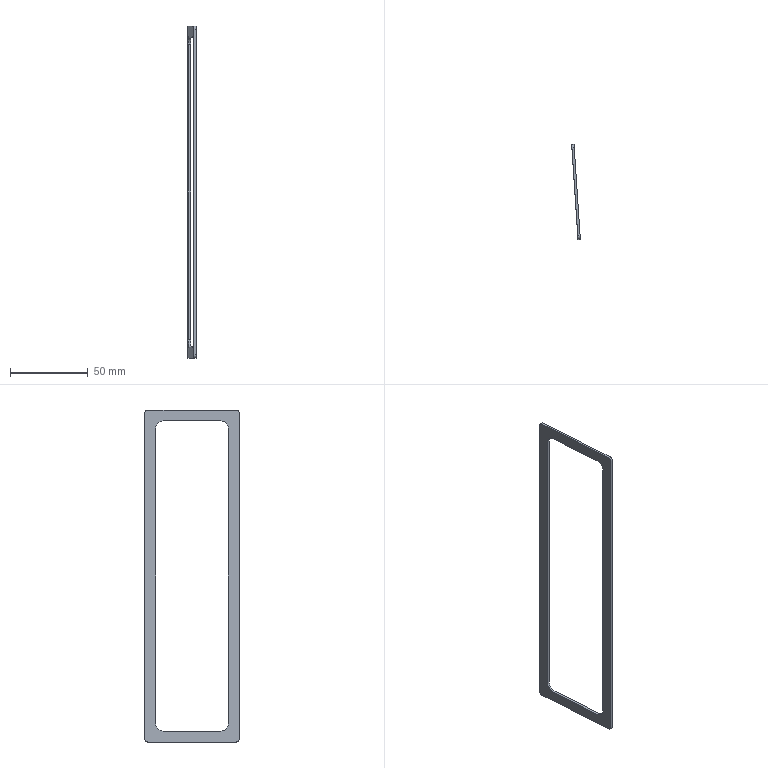Part | SolidWorks | features BaseBody 1 | 1 solid | 18 faces | box 5.536 x 60.965 x 214 mm | volume 5508 mm3 | plane 10 | cylinder 8 | commonest cylinder face diameters 4 x4 10 x4
STEP:
#1=CARTESIAN_POINT('',(-18.857,44.213,71.25));
#2=VERTEX_POINT('',#1);
#3=CARTESIAN_POINT('',(-18.857,44.213,-118.75));
#4=VERTEX_POINT('',#3);
#5=CARTESIAN_POINT('',(-18.857,44.213,-118.75));
#6=DIRECTION('',(0.,0.,-1.));
#7=VECTOR('',#6,1000.);
#8=LINE('',#5,#7);
#9=EDGE_CURVE('',#2,#4,#8,.T.);
#10=ORIENTED_EDGE('',*,*,#9,.F.);
#11=CARTESIAN_POINT('',(-20.353,44.113,71.25));
#12=VERTEX_POINT('',#11);
#13=CARTESIAN_POINT('',(-20.353,44.113,71.25));
#14=DIRECTION('',(0.9978,0.06623,0.));
#15=VECTOR('',#14,1000.);
#16=LINE('',#13,#15);
#17=EDGE_CURVE('',#12,#2,#16,.T.);
#18=ORIENTED_EDGE('',*,*,#17,.F.);
#19=CARTESIAN_POINT('',(-20.353,44.113,-118.75));
#20=VERTEX_POINT('',#19);
#21=CARTESIAN_POINT('',(-20.353,44.113,-118.75));
#22=DIRECTION('',(0.,0.,-1.));
#23=VECTOR('',#22,1000.);
#24=LINE('',#21,#23);
#25=EDGE_CURVE('',#12,#20,#24,.T.);
#26=ORIENTED_EDGE('',*,*,#25,.T.);
#27=CARTESIAN_POINT('',(-20.353,44.113,-118.75));
#28=DIRECTION('',(0.9978,0.06623,0.));
#29=VECTOR('',#28,1000.);
#30=LINE('',#27,#29);
#31=EDGE_CURVE('',#20,#4,#30,.T.);
#32=ORIENTED_EDGE('',*,*,#31,.T.);
#33=EDGE_LOOP('',(#10,#18,#26,#32));
#34=FACE_OUTER_BOUND('',#33,.T.);
#35=CARTESIAN_POINT('',(-20.353,44.113,-118.75));
#36=DIRECTION('',(0.06623,-0.9978,0.));
#37=DIRECTION('',(0.,0.,-1.));
#38=AXIS2_PLACEMENT_3D('',#35,#36,#37);
#39=PLANE('',#38);
#40=ADVANCED_FACE('',(#34),#39,.T.);
#41=CARTESIAN_POINT('',(-18.526,39.224,76.25));
#42=VERTEX_POINT('',#41);
#43=CARTESIAN_POINT('',(-18.526,39.224,71.25));
#44=DIRECTION('',(-0.9978,-0.06623,0.));
#45=DIRECTION('',(0.,0.,-1.));
#46=AXIS2_PLACEMENT_3D('',#43,#44,#45);
#47=CIRCLE('',#46,5.);
#48=EDGE_CURVE('',#42,#2,#47,.T.);
#49=ORIENTED_EDGE('',*,*,#48,.F.);
#50=CARTESIAN_POINT('',(-20.022,39.124,76.25));
#51=VERTEX_POINT('',#50);
#52=CARTESIAN_POINT('',(-20.022,39.124,76.25));
#53=DIRECTION('',(0.9978,0.06623,0.));
#54=VECTOR('',#53,1000.);
#55=LINE('',#52,#54);
#56=EDGE_CURVE('',#51,#42,#55,.T.);
#57=ORIENTED_EDGE('',*,*,#56,.F.);
#58=CARTESIAN_POINT('',(-20.022,39.124,71.25));
#59=DIRECTION('',(-0.9978,-0.06623,0.));
#60=DIRECTION('',(0.,0.,-1.));
#61=AXIS2_PLACEMENT_3D('',#58,#59,#60);
#62=CIRCLE('',#61,5.);
#63=EDGE_CURVE('',#51,#12,#62,.T.);
#64=ORIENTED_EDGE('',*,*,#63,.T.);
#65=ORIENTED_EDGE('',*,*,#17,.T.);
#66=EDGE_LOOP('',(#49,#57,#64,#65));
#67=FACE_OUTER_BOUND('',#66,.T.);
#68=CARTESIAN_POINT('',(-20.022,39.124,71.25));
#69=DIRECTION('',(0.9978,0.06623,0.));
#70=DIRECTION('',(0.,0.,-1.));
#71=AXIS2_PLACEMENT_3D('',#68,#69,#70);
#72=CYLINDRICAL_SURFACE('',#71,5.);
#73=ADVANCED_FACE('',(#67),#72,.F.);
#74=CARTESIAN_POINT('',(-16.075,2.305,76.25));
#75=VERTEX_POINT('',#74);
#76=CARTESIAN_POINT('',(-18.526,39.224,76.25));
#77=DIRECTION('',(-0.06623,0.9978,0.));
#78=VECTOR('',#77,1000.);
#79=LINE('',#76,#78);
#80=EDGE_CURVE('',#75,#42,#79,.T.);
#81=ORIENTED_EDGE('',*,*,#80,.F.);
#82=CARTESIAN_POINT('',(-17.572,2.206,76.25));
#83=VERTEX_POINT('',#82);
#84=CARTESIAN_POINT('',(-17.572,2.206,76.25));
#85=DIRECTION('',(0.9978,0.06623,0.));
#86=VECTOR('',#85,1000.);
#87=LINE('',#84,#86);
#88=EDGE_CURVE('',#83,#75,#87,.T.);
#89=ORIENTED_EDGE('',*,*,#88,.F.);
#90=CARTESIAN_POINT('',(-20.022,39.124,76.25));
#91=DIRECTION('',(-0.06623,0.9978,0.));
#92=VECTOR('',#91,1000.);
#93=LINE('',#90,#92);
#94=EDGE_CURVE('',#83,#51,#93,.T.);
#95=ORIENTED_EDGE('',*,*,#94,.T.);
#96=ORIENTED_EDGE('',*,*,#56,.T.);
#97=EDGE_LOOP('',(#81,#89,#95,#96));
#98=FACE_OUTER_BOUND('',#97,.T.);
#99=CARTESIAN_POINT('',(-20.022,39.124,76.25));
#100=DIRECTION('',(0.,0.,-1.));
#101=DIRECTION('',(-1.,0.,0.));
#102=AXIS2_PLACEMENT_3D('',#99,#100,#101);
#103=PLANE('',#102);
#104=ADVANCED_FACE('',(#98),#103,.T.);
#105=CARTESIAN_POINT('',(-15.744,-2.684,71.25));
#106=VERTEX_POINT('',#105);
#107=CARTESIAN_POINT('',(-16.075,2.305,71.25));
#108=DIRECTION('',(-0.9978,-0.06623,0.));
#109=DIRECTION('',(0.,0.,-1.));
#110=AXIS2_PLACEMENT_3D('',#107,#108,#109);
#111=CIRCLE('',#110,5.);
#112=EDGE_CURVE('',#106,#75,#111,.T.);
#113=ORIENTED_EDGE('',*,*,#112,.F.);
#114=CARTESIAN_POINT('',(-17.241,-2.783,71.25));
#115=VERTEX_POINT('',#114);
#116=CARTESIAN_POINT('',(-17.241,-2.783,71.25));
#117=DIRECTION('',(0.9978,0.06623,0.));
#118=VECTOR('',#117,1000.);
#119=LINE('',#116,#118);
#120=EDGE_CURVE('',#115,#106,#119,.T.);
#121=ORIENTED_EDGE('',*,*,#120,.F.);
#122=CARTESIAN_POINT('',(-17.572,2.206,71.25));
#123=DIRECTION('',(-0.9978,-0.06623,0.));
#124=DIRECTION('',(0.,0.,-1.));
#125=AXIS2_PLACEMENT_3D('',#122,#123,#124);
#126=CIRCLE('',#125,5.);
#127=EDGE_CURVE('',#115,#83,#126,.T.);
#128=ORIENTED_EDGE('',*,*,#127,.T.);
#129=ORIENTED_EDGE('',*,*,#88,.T.);
#130=EDGE_LOOP('',(#113,#121,#128,#129));
#131=FACE_OUTER_BOUND('',#130,.T.);
#132=CARTESIAN_POINT('',(-17.572,2.206,71.25));
#133=DIRECTION('',(0.9978,0.06623,0.));
#134=DIRECTION('',(0.,0.,-1.));
#135=AXIS2_PLACEMENT_3D('',#132,#133,#134);
#136=CYLINDRICAL_SURFACE('',#135,5.);
#137=ADVANCED_FACE('',(#131),#136,.F.);
#138=CARTESIAN_POINT('',(-15.744,-2.684,-118.75));
#139=VERTEX_POINT('',#138);
#140=CARTESIAN_POINT('',(-15.744,-2.684,-118.75));
#141=DIRECTION('',(0.,0.,1.));
#142=VECTOR('',#141,1000.);
#143=LINE('',#140,#142);
#144=EDGE_CURVE('',#139,#106,#143,.T.);
#145=ORIENTED_EDGE('',*,*,#144,.F.);
#146=CARTESIAN_POINT('',(-17.241,-2.783,-118.75));
#147=VERTEX_POINT('',#146);
#148=CARTESIAN_POINT('',(-17.241,-2.783,-118.75));
#149=DIRECTION('',(0.9978,0.06623,0.));
#150=VECTOR('',#149,1000.);
#151=LINE('',#148,#150);
#152=EDGE_CURVE('',#147,#139,#151,.T.);
#153=ORIENTED_EDGE('',*,*,#152,.F.);
#154=CARTESIAN_POINT('',(-17.241,-2.783,-118.75));
#155=DIRECTION('',(0.,0.,1.));
#156=VECTOR('',#155,1000.);
#157=LINE('',#154,#156);
#158=EDGE_CURVE('',#147,#115,#157,.T.);
#159=ORIENTED_EDGE('',*,*,#158,.T.);
#160=ORIENTED_EDGE('',*,*,#120,.T.);
#161=EDGE_LOOP('',(#145,#153,#159,#160));
#162=FACE_OUTER_BOUND('',#161,.T.);
#163=CARTESIAN_POINT('',(-17.241,-2.783,-118.75));
#164=DIRECTION('',(-0.06623,0.9978,0.));
#165=DIRECTION('',(0.,0.,1.));
#166=AXIS2_PLACEMENT_3D('',#163,#164,#165);
#167=PLANE('',#166);
#168=ADVANCED_FACE('',(#162),#167,.T.);
#169=CARTESIAN_POINT('',(-16.075,2.305,-123.75));
#170=VERTEX_POINT('',#169);
#171=CARTESIAN_POINT('',(-16.075,2.305,-118.75));
#172=DIRECTION('',(-0.9978,-0.06623,0.));
#173=DIRECTION('',(0.,0.,-1.));
#174=AXIS2_PLACEMENT_3D('',#171,#172,#173);
#175=CIRCLE('',#174,5.);
#176=EDGE_CURVE('',#170,#139,#175,.T.);
#177=ORIENTED_EDGE('',*,*,#176,.F.);
#178=CARTESIAN_POINT('',(-17.572,2.206,-123.75));
#179=VERTEX_POINT('',#178);
#180=CARTESIAN_POINT('',(-17.572,2.206,-123.75));
#181=DIRECTION('',(0.9978,0.06623,0.));
#182=VECTOR('',#181,1000.);
#183=LINE('',#180,#182);
#184=EDGE_CURVE('',#179,#170,#183,.T.);
#185=ORIENTED_EDGE('',*,*,#184,.F.);
#186=CARTESIAN_POINT('',(-17.572,2.206,-118.75));
#187=DIRECTION('',(-0.9978,-0.06623,0.));
#188=DIRECTION('',(0.,0.,-1.));
#189=AXIS2_PLACEMENT_3D('',#186,#187,#188);
#190=CIRCLE('',#189,5.);
#191=EDGE_CURVE('',#179,#147,#190,.T.);
#192=ORIENTED_EDGE('',*,*,#191,.T.);
#193=ORIENTED_EDGE('',*,*,#152,.T.);
#194=EDGE_LOOP('',(#177,#185,#192,#193));
#195=FACE_OUTER_BOUND('',#194,.T.);
#196=CARTESIAN_POINT('',(-17.572,2.206,-118.75));
#197=DIRECTION('',(0.9978,0.06623,0.));
#198=DIRECTION('',(0.,0.,-1.));
#199=AXIS2_PLACEMENT_3D('',#196,#197,#198);
#200=CYLINDRICAL_SURFACE('',#199,5.);
#201=ADVANCED_FACE('',(#195),#200,.F.);
#202=CARTESIAN_POINT('',(-18.526,39.224,-123.75));
#203=VERTEX_POINT('',#202);
#204=CARTESIAN_POINT('',(-18.526,39.224,-123.75));
#205=DIRECTION('',(0.06623,-0.9978,0.));
#206=VECTOR('',#205,1000.);
#207=LINE('',#204,#206);
#208=EDGE_CURVE('',#203,#170,#207,.T.);
#209=ORIENTED_EDGE('',*,*,#208,.F.);
#210=CARTESIAN_POINT('',(-20.022,39.124,-123.75));
#211=VERTEX_POINT('',#210);
#212=CARTESIAN_POINT('',(-20.022,39.124,-123.75));
#213=DIRECTION('',(0.9978,0.06623,0.));
#214=VECTOR('',#213,1000.);
#215=LINE('',#212,#214);
#216=EDGE_CURVE('',#211,#203,#215,.T.);
#217=ORIENTED_EDGE('',*,*,#216,.F.);
#218=CARTESIAN_POINT('',(-20.022,39.124,-123.75));
#219=DIRECTION('',(0.06623,-0.9978,0.));
#220=VECTOR('',#219,1000.);
#221=LINE('',#218,#220);
#222=EDGE_CURVE('',#211,#179,#221,.T.);
#223=ORIENTED_EDGE('',*,*,#222,.T.);
#224=ORIENTED_EDGE('',*,*,#184,.T.);
#225=EDGE_LOOP('',(#209,#217,#223,#224));
#226=FACE_OUTER_BOUND('',#225,.T.);
#227=CARTESIAN_POINT('',(-20.022,39.124,-123.75));
#228=DIRECTION('',(0.,0.,1.));
#229=DIRECTION('',(1.,0.,0.));
#230=AXIS2_PLACEMENT_3D('',#227,#228,#229);
#231=PLANE('',#230);
#232=ADVANCED_FACE('',(#226),#231,.T.);
#233=CARTESIAN_POINT('',(-18.526,39.224,-118.75));
#234=DIRECTION('',(-0.9978,-0.06623,0.));
#235=DIRECTION('',(0.,0.,1.));
#236=AXIS2_PLACEMENT_3D('',#233,#234,#235);
#237=CIRCLE('',#236,5.);
#238=EDGE_CURVE('',#4,#203,#237,.T.);
#239=ORIENTED_EDGE('',*,*,#238,.F.);
#240=ORIENTED_EDGE('',*,*,#31,.F.);
#241=CARTESIAN_POINT('',(-20.022,39.124,-118.75));
#242=DIRECTION('',(-0.9978,-0.06623,0.));
#243=DIRECTION('',(0.,0.,1.));
#244=AXIS2_PLACEMENT_3D('',#241,#242,#243);
#245=CIRCLE('',#244,5.);
#246=EDGE_CURVE('',#20,#211,#245,.T.);
#247=ORIENTED_EDGE('',*,*,#246,.T.);
#248=ORIENTED_EDGE('',*,*,#216,.T.);
#249=EDGE_LOOP('',(#239,#240,#247,#248));
#250=FACE_OUTER_BOUND('',#249,.T.);
#251=CARTESIAN_POINT('',(-20.022,39.124,-118.75));
#252=DIRECTION('',(0.9978,0.06623,0.));
#253=DIRECTION('',(0.,0.,-1.));
#254=AXIS2_PLACEMENT_3D('',#251,#252,#253);
#255=CYLINDRICAL_SURFACE('',#254,5.);
#256=ADVANCED_FACE('',(#250),#255,.F.);
#257=CARTESIAN_POINT('',(-15.28,-9.669,-128.75));
#258=VERTEX_POINT('',#257);
#259=CARTESIAN_POINT('',(-15.28,-9.669,81.25));
#260=VERTEX_POINT('',#259);
#261=CARTESIAN_POINT('',(-15.28,-9.669,-128.75));
#262=DIRECTION('',(0.,0.,1.));
#263=VECTOR('',#262,1000.);
#264=LINE('',#261,#263);
#265=EDGE_CURVE('',#258,#260,#264,.T.);
#266=ORIENTED_EDGE('',*,*,#265,.T.);
#267=CARTESIAN_POINT('',(-16.777,-9.768,81.25));
#268=VERTEX_POINT('',#267);
#269=CARTESIAN_POINT('',(-16.777,-9.768,81.25));
#270=DIRECTION('',(0.9978,0.06623,0.));
#271=VECTOR('',#270,1000.);
#272=LINE('',#269,#271);
#273=EDGE_CURVE('',#268,#260,#272,.T.);
#274=ORIENTED_EDGE('',*,*,#273,.F.);
#275=CARTESIAN_POINT('',(-16.777,-9.768,-128.75));
#276=VERTEX_POINT('',#275);
#277=CARTESIAN_POINT('',(-16.777,-9.768,-128.75));
#278=DIRECTION('',(0.,0.,1.));
#279=VECTOR('',#278,1000.);
#280=LINE('',#277,#279);
#281=EDGE_CURVE('',#276,#268,#280,.T.);
#282=ORIENTED_EDGE('',*,*,#281,.F.);
#283=CARTESIAN_POINT('',(-16.777,-9.768,-128.75));
#284=DIRECTION('',(0.9978,0.06623,0.));
#285=VECTOR('',#284,1000.);
#286=LINE('',#283,#285);
#287=EDGE_CURVE('',#276,#258,#286,.T.);
#288=ORIENTED_EDGE('',*,*,#287,.T.);
#289=EDGE_LOOP('',(#266,#274,#282,#288));
#290=FACE_OUTER_BOUND('',#289,.T.);
#291=CARTESIAN_POINT('',(-16.777,-9.768,-128.75));
#292=DIRECTION('',(-0.06623,0.9978,0.));
#293=DIRECTION('',(0.,0.,1.));
#294=AXIS2_PLACEMENT_3D('',#291,#292,#293);
#295=PLANE('',#294);
#296=ADVANCED_FACE('',(#290),#295,.F.);
#297=CARTESIAN_POINT('',(-15.413,-7.673,-130.75));
#298=VERTEX_POINT('',#297);
#299=CARTESIAN_POINT('',(-15.413,-7.673,-128.75));
#300=DIRECTION('',(-0.9978,-0.06623,0.));
#301=DIRECTION('',(0.,0.,-1.));
#302=AXIS2_PLACEMENT_3D('',#299,#300,#301);
#303=CIRCLE('',#302,2.);
#304=EDGE_CURVE('',#298,#258,#303,.T.);
#305=ORIENTED_EDGE('',*,*,#304,.T.);
#306=ORIENTED_EDGE('',*,*,#287,.F.);
#307=CARTESIAN_POINT('',(-16.91,-7.772,-130.75));
#308=VERTEX_POINT('',#307);
#309=CARTESIAN_POINT('',(-16.91,-7.772,-128.75));
#310=DIRECTION('',(-0.9978,-0.06623,0.));
#311=DIRECTION('',(0.,0.,-1.));
#312=AXIS2_PLACEMENT_3D('',#309,#310,#311);
#313=CIRCLE('',#312,2.);
#314=EDGE_CURVE('',#308,#276,#313,.T.);
#315=ORIENTED_EDGE('',*,*,#314,.F.);
#316=CARTESIAN_POINT('',(-16.91,-7.772,-130.75));
#317=DIRECTION('',(0.9978,0.06623,0.));
#318=VECTOR('',#317,1000.);
#319=LINE('',#316,#318);
#320=EDGE_CURVE('',#308,#298,#319,.T.);
#321=ORIENTED_EDGE('',*,*,#320,.T.);
#322=EDGE_LOOP('',(#305,#306,#315,#321));
#323=FACE_OUTER_BOUND('',#322,.T.);
#324=CARTESIAN_POINT('',(-16.91,-7.772,-128.75));
#325=DIRECTION('',(0.9978,0.06623,0.));
#326=DIRECTION('',(0.,0.,-1.));
#327=AXIS2_PLACEMENT_3D('',#324,#325,#326);
#328=CYLINDRICAL_SURFACE('',#327,2.);
#329=ADVANCED_FACE('',(#323),#328,.T.);
#330=CARTESIAN_POINT('',(-19.188,49.202,-130.75));
#331=VERTEX_POINT('',#330);
#332=CARTESIAN_POINT('',(-19.188,49.202,-130.75));
#333=DIRECTION('',(0.06623,-0.9978,0.));
#334=VECTOR('',#333,1000.);
#335=LINE('',#332,#334);
#336=EDGE_CURVE('',#331,#298,#335,.T.);
#337=ORIENTED_EDGE('',*,*,#336,.T.);
#338=ORIENTED_EDGE('',*,*,#320,.F.);
#339=CARTESIAN_POINT('',(-20.684,49.102,-130.75));
#340=VERTEX_POINT('',#339);
#341=CARTESIAN_POINT('',(-20.684,49.102,-130.75));
#342=DIRECTION('',(0.06623,-0.9978,0.));
#343=VECTOR('',#342,1000.);
#344=LINE('',#341,#343);
#345=EDGE_CURVE('',#340,#308,#344,.T.);
#346=ORIENTED_EDGE('',*,*,#345,.F.);
#347=CARTESIAN_POINT('',(-20.684,49.102,-130.75));
#348=DIRECTION('',(0.9978,0.06623,0.));
#349=VECTOR('',#348,1000.);
#350=LINE('',#347,#349);
#351=EDGE_CURVE('',#340,#331,#350,.T.);
#352=ORIENTED_EDGE('',*,*,#351,.T.);
#353=EDGE_LOOP('',(#337,#338,#346,#352));
#354=FACE_OUTER_BOUND('',#353,.T.);
#355=CARTESIAN_POINT('',(-20.684,49.102,-130.75));
#356=DIRECTION('',(0.,0.,1.));
#357=DIRECTION('',(1.,0.,0.));
#358=AXIS2_PLACEMENT_3D('',#355,#356,#357);
#359=PLANE('',#358);
#360=ADVANCED_FACE('',(#354),#359,.F.);
#361=CARTESIAN_POINT('',(-19.32,51.197,-128.75));
#362=VERTEX_POINT('',#361);
#363=CARTESIAN_POINT('',(-19.188,49.202,-128.75));
#364=DIRECTION('',(-0.9978,-0.06623,0.));
#365=DIRECTION('',(0.,0.,-1.));
#366=AXIS2_PLACEMENT_3D('',#363,#364,#365);
#367=CIRCLE('',#366,2.);
#368=EDGE_CURVE('',#362,#331,#367,.T.);
#369=ORIENTED_EDGE('',*,*,#368,.T.);
#370=ORIENTED_EDGE('',*,*,#351,.F.);
#371=CARTESIAN_POINT('',(-20.817,51.098,-128.75));
#372=VERTEX_POINT('',#371);
#373=CARTESIAN_POINT('',(-20.684,49.102,-128.75));
#374=DIRECTION('',(-0.9978,-0.06623,0.));
#375=DIRECTION('',(0.,0.,-1.));
#376=AXIS2_PLACEMENT_3D('',#373,#374,#375);
#377=CIRCLE('',#376,2.);
#378=EDGE_CURVE('',#372,#340,#377,.T.);
#379=ORIENTED_EDGE('',*,*,#378,.F.);
#380=CARTESIAN_POINT('',(-20.817,51.098,-128.75));
#381=DIRECTION('',(0.9978,0.06623,0.));
#382=VECTOR('',#381,1000.);
#383=LINE('',#380,#382);
#384=EDGE_CURVE('',#372,#362,#383,.T.);
#385=ORIENTED_EDGE('',*,*,#384,.T.);
#386=EDGE_LOOP('',(#369,#370,#379,#385));
#387=FACE_OUTER_BOUND('',#386,.T.);
#388=CARTESIAN_POINT('',(-20.684,49.102,-128.75));
#389=DIRECTION('',(0.9978,0.06623,0.));
#390=DIRECTION('',(0.,0.,-1.));
#391=AXIS2_PLACEMENT_3D('',#388,#389,#390);
#392=CYLINDRICAL_SURFACE('',#391,2.);
#393=ADVANCED_FACE('',(#387),#392,.T.);
#394=CARTESIAN_POINT('',(-19.32,51.197,81.25));
#395=VERTEX_POINT('',#394);
#396=CARTESIAN_POINT('',(-19.32,51.197,-128.75));
#397=DIRECTION('',(0.,0.,-1.));
#398=VECTOR('',#397,1000.);
#399=LINE('',#396,#398);
#400=EDGE_CURVE('',#395,#362,#399,.T.);
#401=ORIENTED_EDGE('',*,*,#400,.T.);
#402=ORIENTED_EDGE('',*,*,#384,.F.);
#403=CARTESIAN_POINT('',(-20.817,51.098,81.25));
#404=VERTEX_POINT('',#403);
#405=CARTESIAN_POINT('',(-20.817,51.098,-128.75));
#406=DIRECTION('',(0.,0.,-1.));
#407=VECTOR('',#406,1000.);
#408=LINE('',#405,#407);
#409=EDGE_CURVE('',#404,#372,#408,.T.);
#410=ORIENTED_EDGE('',*,*,#409,.F.);
#411=CARTESIAN_POINT('',(-20.817,51.098,81.25));
#412=DIRECTION('',(0.9978,0.06623,0.));
#413=VECTOR('',#412,1000.);
#414=LINE('',#411,#413);
#415=EDGE_CURVE('',#404,#395,#414,.T.);
#416=ORIENTED_EDGE('',*,*,#415,.T.);
#417=EDGE_LOOP('',(#401,#402,#410,#416));
#418=FACE_OUTER_BOUND('',#417,.T.);
#419=CARTESIAN_POINT('',(-20.817,51.098,-128.75));
#420=DIRECTION('',(0.06623,-0.9978,0.));
#421=DIRECTION('',(0.,0.,-1.));
#422=AXIS2_PLACEMENT_3D('',#419,#420,#421);
#423=PLANE('',#422);
#424=ADVANCED_FACE('',(#418),#423,.F.);
#425=CARTESIAN_POINT('',(-19.188,49.202,83.25));
#426=VERTEX_POINT('',#425);
#427=CARTESIAN_POINT('',(-19.188,49.202,81.25));
#428=DIRECTION('',(-0.9978,-0.06623,0.));
#429=DIRECTION('',(0.,0.,-1.));
#430=AXIS2_PLACEMENT_3D('',#427,#428,#429);
#431=CIRCLE('',#430,2.);
#432=EDGE_CURVE('',#426,#395,#431,.T.);
#433=ORIENTED_EDGE('',*,*,#432,.T.);
#434=ORIENTED_EDGE('',*,*,#415,.F.);
#435=CARTESIAN_POINT('',(-20.684,49.102,83.25));
#436=VERTEX_POINT('',#435);
#437=CARTESIAN_POINT('',(-20.684,49.102,81.25));
#438=DIRECTION('',(-0.9978,-0.06623,0.));
#439=DIRECTION('',(0.,0.,-1.));
#440=AXIS2_PLACEMENT_3D('',#437,#438,#439);
#441=CIRCLE('',#440,2.);
#442=EDGE_CURVE('',#436,#404,#441,.T.);
#443=ORIENTED_EDGE('',*,*,#442,.F.);
#444=CARTESIAN_POINT('',(-20.684,49.102,83.25));
#445=DIRECTION('',(0.9978,0.06623,0.));
#446=VECTOR('',#445,1000.);
#447=LINE('',#444,#446);
#448=EDGE_CURVE('',#436,#426,#447,.T.);
#449=ORIENTED_EDGE('',*,*,#448,.T.);
#450=EDGE_LOOP('',(#433,#434,#443,#449));
#451=FACE_OUTER_BOUND('',#450,.T.);
#452=CARTESIAN_POINT('',(-20.684,49.102,81.25));
#453=DIRECTION('',(0.9978,0.06623,0.));
#454=DIRECTION('',(0.,0.,-1.));
#455=AXIS2_PLACEMENT_3D('',#452,#453,#454);
#456=CYLINDRICAL_SURFACE('',#455,2.);
#457=ADVANCED_FACE('',(#451),#456,.T.);
#458=CARTESIAN_POINT('',(-15.413,-7.673,83.25));
#459=VERTEX_POINT('',#458);
#460=CARTESIAN_POINT('',(-19.188,49.202,83.25));
#461=DIRECTION('',(-0.06623,0.9978,0.));
#462=VECTOR('',#461,1000.);
#463=LINE('',#460,#462);
#464=EDGE_CURVE('',#459,#426,#463,.T.);
#465=ORIENTED_EDGE('',*,*,#464,.T.);
#466=ORIENTED_EDGE('',*,*,#448,.F.);
#467=CARTESIAN_POINT('',(-16.91,-7.772,83.25));
#468=VERTEX_POINT('',#467);
#469=CARTESIAN_POINT('',(-20.684,49.102,83.25));
#470=DIRECTION('',(-0.06623,0.9978,0.));
#471=VECTOR('',#470,1000.);
#472=LINE('',#469,#471);
#473=EDGE_CURVE('',#468,#436,#472,.T.);
#474=ORIENTED_EDGE('',*,*,#473,.F.);
#475=CARTESIAN_POINT('',(-16.91,-7.772,83.25));
#476=DIRECTION('',(0.9978,0.06623,0.));
#477=VECTOR('',#476,1000.);
#478=LINE('',#475,#477);
#479=EDGE_CURVE('',#468,#459,#478,.T.);
#480=ORIENTED_EDGE('',*,*,#479,.T.);
#481=EDGE_LOOP('',(#465,#466,#474,#480));
#482=FACE_OUTER_BOUND('',#481,.T.);
#483=CARTESIAN_POINT('',(-20.684,49.102,83.25));
#484=DIRECTION('',(0.,0.,-1.));
#485=DIRECTION('',(-1.,0.,0.));
#486=AXIS2_PLACEMENT_3D('',#483,#484,#485);
#487=PLANE('',#486);
#488=ADVANCED_FACE('',(#482),#487,.F.);
#489=CARTESIAN_POINT('',(-15.413,-7.673,81.25));
#490=DIRECTION('',(-0.9978,-0.06623,0.));
#491=DIRECTION('',(0.,0.,-1.));
#492=AXIS2_PLACEMENT_3D('',#489,#490,#491);
#493=CIRCLE('',#492,2.);
#494=EDGE_CURVE('',#260,#459,#493,.T.);
#495=ORIENTED_EDGE('',*,*,#494,.T.);
#496=ORIENTED_EDGE('',*,*,#479,.F.);
#497=CARTESIAN_POINT('',(-16.91,-7.772,81.25));
#498=DIRECTION('',(-0.9978,-0.06623,0.));
#499=DIRECTION('',(0.,0.,-1.));
#500=AXIS2_PLACEMENT_3D('',#497,#498,#499);
#501=CIRCLE('',#500,2.);
#502=EDGE_CURVE('',#268,#468,#501,.T.);
#503=ORIENTED_EDGE('',*,*,#502,.F.);
#504=ORIENTED_EDGE('',*,*,#273,.T.);
#505=EDGE_LOOP('',(#495,#496,#503,#504));
#506=FACE_OUTER_BOUND('',#505,.T.);
#507=CARTESIAN_POINT('',(-16.91,-7.772,81.25));
#508=DIRECTION('',(0.9978,0.06623,0.));
#509=DIRECTION('',(0.,0.,-1.));
#510=AXIS2_PLACEMENT_3D('',#507,#508,#509);
#511=CYLINDRICAL_SURFACE('',#510,2.);
#512=ADVANCED_FACE('',(#506),#511,.T.);
#513=ORIENTED_EDGE('',*,*,#9,.T.);
#514=ORIENTED_EDGE('',*,*,#238,.T.);
#515=ORIENTED_EDGE('',*,*,#208,.T.);
#516=ORIENTED_EDGE('',*,*,#176,.T.);
#517=ORIENTED_EDGE('',*,*,#144,.T.);
#518=ORIENTED_EDGE('',*,*,#112,.T.);
#519=ORIENTED_EDGE('',*,*,#80,.T.);
#520=ORIENTED_EDGE('',*,*,#48,.T.);
#521=EDGE_LOOP('',(#513,#514,#515,#516,#517,#518,#519,#520));
#522=FACE_BOUND('',#521,.T.);
#523=ORIENTED_EDGE('',*,*,#494,.F.);
#524=ORIENTED_EDGE('',*,*,#265,.F.);
#525=ORIENTED_EDGE('',*,*,#304,.F.);
#526=ORIENTED_EDGE('',*,*,#336,.F.);
#527=ORIENTED_EDGE('',*,*,#368,.F.);
#528=ORIENTED_EDGE('',*,*,#400,.F.);
#529=ORIENTED_EDGE('',*,*,#432,.F.);
#530=ORIENTED_EDGE('',*,*,#464,.F.);
#531=EDGE_LOOP('',(#523,#524,#525,#526,#527,#528,#529,#530));
#532=FACE_OUTER_BOUND('',#531,.T.);
#533=CARTESIAN_POINT('',(-15.413,-7.673,81.25));
#534=DIRECTION('',(0.9978,0.06623,0.));
#535=DIRECTION('',(0.,0.,-1.));
#536=AXIS2_PLACEMENT_3D('',#533,#534,#535);
#537=PLANE('',#536);
#538=ADVANCED_FACE('',(#522,#532),#537,.T.);
#539=ORIENTED_EDGE('',*,*,#246,.F.);
#540=ORIENTED_EDGE('',*,*,#25,.F.);
#541=ORIENTED_EDGE('',*,*,#63,.F.);
#542=ORIENTED_EDGE('',*,*,#94,.F.);
#543=ORIENTED_EDGE('',*,*,#127,.F.);
#544=ORIENTED_EDGE('',*,*,#158,.F.);
#545=ORIENTED_EDGE('',*,*,#191,.F.);
#546=ORIENTED_EDGE('',*,*,#222,.F.);
#547=EDGE_LOOP('',(#539,#540,#541,#542,#543,#544,#545,#546));
#548=FACE_BOUND('',#547,.T.);
#549=ORIENTED_EDGE('',*,*,#502,.T.);
#550=ORIENTED_EDGE('',*,*,#473,.T.);
#551=ORIENTED_EDGE('',*,*,#442,.T.);
#552=ORIENTED_EDGE('',*,*,#409,.T.);
#553=ORIENTED_EDGE('',*,*,#378,.T.);
#554=ORIENTED_EDGE('',*,*,#345,.T.);
#555=ORIENTED_EDGE('',*,*,#314,.T.);
#556=ORIENTED_EDGE('',*,*,#281,.T.);
#557=EDGE_LOOP('',(#549,#550,#551,#552,#553,#554,#555,#556));
#558=FACE_OUTER_BOUND('',#557,.T.);
#559=CARTESIAN_POINT('',(-16.91,-7.772,81.25));
#560=DIRECTION('',(0.9978,0.06623,0.));
#561=DIRECTION('',(0.,0.,-1.));
#562=AXIS2_PLACEMENT_3D('',#559,#560,#561);
#563=PLANE('',#562);
#564=ADVANCED_FACE('',(#548,#558),#563,.F.);
#565=CLOSED_SHELL('',(#40,#73,#104,#137,#168,#201,#232,#256,#296,#329,#360,#393,#424,#457,#488,#512,#538,#564));
#566=MANIFOLD_SOLID_BREP('',#565);
#567=CARTESIAN_POINT('',(0.,0.,0.));
#568=DIRECTION('',(0.,0.,1.));
#569=DIRECTION('',(1.,0.,0.));
#570=AXIS2_PLACEMENT_3D('',#567,#568,#569);
#571=(LENGTH_UNIT()NAMED_UNIT(*)SI_UNIT(.MILLI.,.METRE.));
#572=UNCERTAINTY_MEASURE_WITH_UNIT(LENGTH_MEASURE(0.00001),#571,'','');
#573=(NAMED_UNIT(*)PLANE_ANGLE_UNIT()SI_UNIT($,.RADIAN.));
#574=(NAMED_UNIT(*)SI_UNIT($,.STERADIAN.)SOLID_ANGLE_UNIT());
#575=(GEOMETRIC_REPRESENTATION_CONTEXT(3)GLOBAL_UNCERTAINTY_ASSIGNED_CONTEXT((#572))GLOBAL_UNIT_ASSIGNED_CONTEXT((#571,#573,#574))REPRESENTATION_CONTEXT('',''));
#576=ADVANCED_BREP_SHAPE_REPRESENTATION('',(#566,#570),#575);